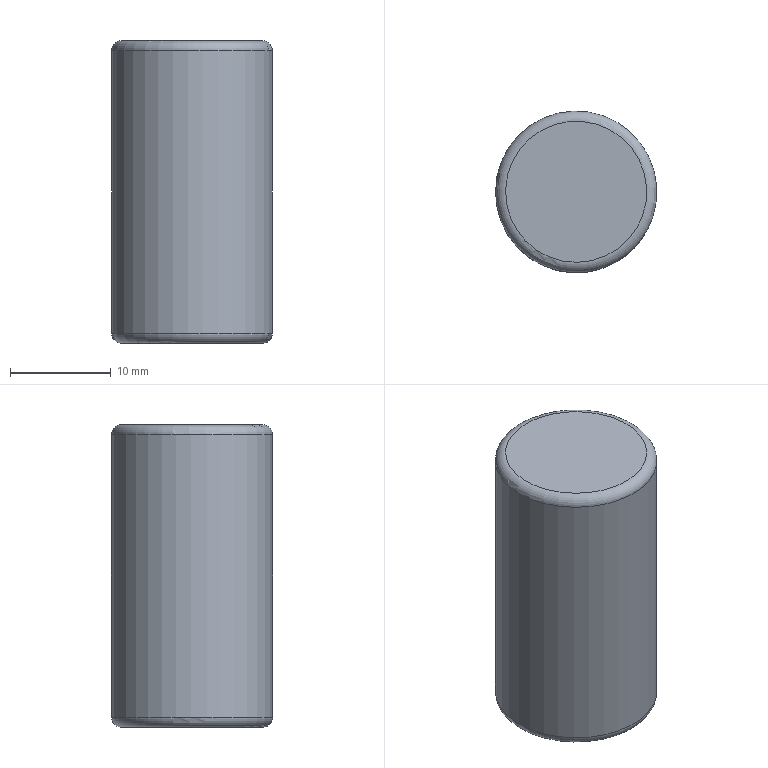Part | STEP file | solid 174 | 1 solid | 5 faces | box 16 x 16 x 30 mm | volume 6011 mm3 | plane 2 | torus 2 | cylinder 1 | commonest cylinder face diameters 16 x1